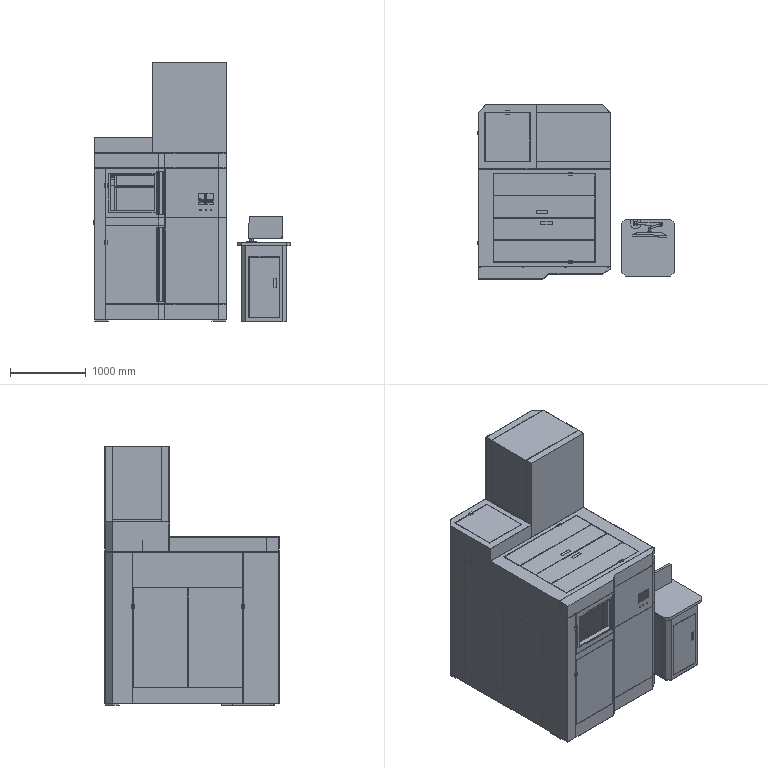Part | SolidWorks | features CompositeCurve 2 | 144 solids | 3204 faces | volume 140729091 mm3 | plane 1809 | cylinder 1389 | cone 4 | spline 2 | commonest cylinder face diameters 9 x622 6 x130 10 x114 7 x106 5 x98 5.5 x88